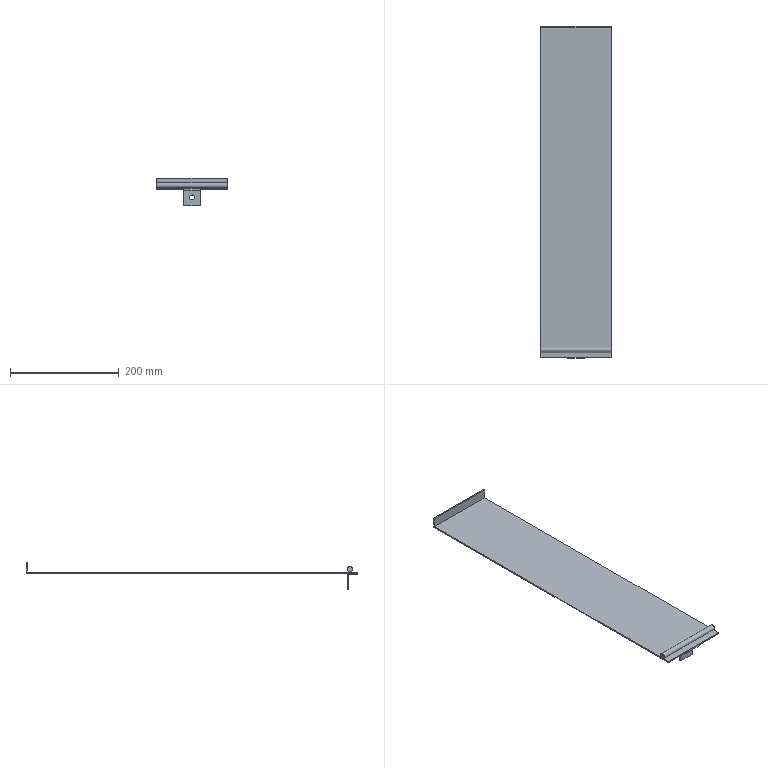Part | NX | features solid 2 | 1 solid | 17 faces | box 130 x 610 x 50 mm | volume 201020 mm3 | plane 15 | cylinder 2 | commonest cylinder face diameters 9 x1 10 x1
STEP:
#1=CARTESIAN_POINT('',(65.,-100.,-520.));
#2=VERTEX_POINT('',#1);
#3=CARTESIAN_POINT('',(65.,-710.,-520.));
#4=VERTEX_POINT('',#3);
#5=CARTESIAN_POINT('',(65.,20.,-520.));
#6=DIRECTION('',(0.,-1.,0.));
#7=VECTOR('',#6,1000.);
#8=LINE('',#5,#7);
#9=EDGE_CURVE('',#2,#4,#8,.T.);
#10=ORIENTED_EDGE('',*,*,#9,.F.);
#11=CARTESIAN_POINT('',(195.,-100.,-520.));
#12=VERTEX_POINT('',#11);
#13=CARTESIAN_POINT('',(365.,-100.,-520.));
#14=DIRECTION('',(1.,0.,0.));
#15=VECTOR('',#14,1000.);
#16=LINE('',#13,#15);
#17=EDGE_CURVE('',#12,#2,#16,.F.);
#18=ORIENTED_EDGE('',*,*,#17,.F.);
#19=CARTESIAN_POINT('',(195.,-710.,-520.));
#20=VERTEX_POINT('',#19);
#21=CARTESIAN_POINT('',(195.,-690.,-520.));
#22=DIRECTION('',(0.,-1.,0.));
#23=VECTOR('',#22,1000.);
#24=LINE('',#21,#23);
#25=EDGE_CURVE('',#12,#20,#24,.T.);
#26=ORIENTED_EDGE('',*,*,#25,.T.);
#27=CARTESIAN_POINT('',(145.,-710.,-520.));
#28=VERTEX_POINT('',#27);
#29=CARTESIAN_POINT('',(1630.,-710.,-520.));
#30=DIRECTION('',(-1.,0.,0.));
#31=VECTOR('',#30,1000.);
#32=LINE('',#29,#31);
#33=EDGE_CURVE('',#20,#28,#32,.T.);
#34=ORIENTED_EDGE('',*,*,#33,.T.);
#35=CARTESIAN_POINT('',(145.,-690.,-520.));
#36=VERTEX_POINT('',#35);
#37=CARTESIAN_POINT('',(145.,-690.,-520.));
#38=DIRECTION('',(0.,-1.,0.));
#39=VECTOR('',#38,1000.);
#40=LINE('',#37,#39);
#41=EDGE_CURVE('',#28,#36,#40,.F.);
#42=ORIENTED_EDGE('',*,*,#41,.T.);
#43=CARTESIAN_POINT('',(115.,-690.,-520.));
#44=VERTEX_POINT('',#43);
#45=CARTESIAN_POINT('',(155.,-690.,-520.));
#46=DIRECTION('',(-1.,0.,0.));
#47=VECTOR('',#46,1000.);
#48=LINE('',#45,#47);
#49=EDGE_CURVE('',#36,#44,#48,.T.);
#50=ORIENTED_EDGE('',*,*,#49,.T.);
#51=CARTESIAN_POINT('',(115.,-710.,-520.));
#52=VERTEX_POINT('',#51);
#53=CARTESIAN_POINT('',(115.,-690.,-520.));
#54=DIRECTION('',(0.,-1.,0.));
#55=VECTOR('',#54,1000.);
#56=LINE('',#53,#55);
#57=EDGE_CURVE('',#44,#52,#56,.T.);
#58=ORIENTED_EDGE('',*,*,#57,.T.);
#59=CARTESIAN_POINT('',(1630.,-710.,-520.));
#60=DIRECTION('',(-1.,0.,0.));
#61=VECTOR('',#60,1000.);
#62=LINE('',#59,#61);
#63=EDGE_CURVE('',#52,#4,#62,.T.);
#64=ORIENTED_EDGE('',*,*,#63,.T.);
#65=EDGE_LOOP('',(#10,#18,#26,#34,#42,#50,#58,#64));
#66=FACE_BOUND('',#65,.T.);
#67=CARTESIAN_POINT('',(365.,-10.,-520.));
#68=DIRECTION('',(0.,0.,-1.));
#69=DIRECTION('',(-1.,0.,0.));
#70=AXIS2_PLACEMENT_3D('',#67,#68,#69);
#71=PLANE('',#70);
#72=ADVANCED_FACE('',(#66),#71,.T.);
#73=CARTESIAN_POINT('',(65.,-102.3,-517.7));
#74=VERTEX_POINT('',#73);
#75=CARTESIAN_POINT('',(65.,-694.005,-517.7));
#76=VERTEX_POINT('',#75);
#77=CARTESIAN_POINT('',(65.,20.,-517.7));
#78=DIRECTION('',(0.,-1.,0.));
#79=VECTOR('',#78,1000.);
#80=LINE('',#77,#79);
#81=EDGE_CURVE('',#74,#76,#80,.T.);
#82=ORIENTED_EDGE('',*,*,#81,.F.);
#83=CARTESIAN_POINT('',(65.,-102.3,-500.));
#84=VERTEX_POINT('',#83);
#85=CARTESIAN_POINT('',(65.,-102.3,-520.));
#86=DIRECTION('',(0.,0.,-1.));
#87=VECTOR('',#86,1000.);
#88=LINE('',#85,#87);
#89=EDGE_CURVE('',#74,#84,#88,.F.);
#90=ORIENTED_EDGE('',*,*,#89,.T.);
#91=CARTESIAN_POINT('',(65.,-100.,-500.));
#92=VERTEX_POINT('',#91);
#93=CARTESIAN_POINT('',(65.,-92.3,-500.));
#94=DIRECTION('',(0.,1.,0.));
#95=VECTOR('',#94,1000.);
#96=LINE('',#93,#95);
#97=EDGE_CURVE('',#92,#84,#96,.F.);
#98=ORIENTED_EDGE('',*,*,#97,.F.);
#99=CARTESIAN_POINT('',(65.,-100.,-520.));
#100=DIRECTION('',(0.,0.,-1.));
#101=VECTOR('',#100,1000.);
#102=LINE('',#99,#101);
#103=EDGE_CURVE('',#2,#92,#102,.F.);
#104=ORIENTED_EDGE('',*,*,#103,.F.);
#105=ORIENTED_EDGE('',*,*,#9,.T.);
#106=CARTESIAN_POINT('',(65.,-710.,-517.7));
#107=VERTEX_POINT('',#106);
#108=CARTESIAN_POINT('',(65.,-710.,-520.));
#109=DIRECTION('',(0.,0.,1.));
#110=VECTOR('',#109,1000.);
#111=LINE('',#108,#110);
#112=EDGE_CURVE('',#4,#107,#111,.T.);
#113=ORIENTED_EDGE('',*,*,#112,.T.);
#114=CARTESIAN_POINT('',(65.,-695.995,-517.7));
#115=VERTEX_POINT('',#114);
#116=CARTESIAN_POINT('',(65.,20.,-517.7));
#117=DIRECTION('',(0.,-1.,0.));
#118=VECTOR('',#117,1000.);
#119=LINE('',#116,#118);
#120=EDGE_CURVE('',#115,#107,#119,.T.);
#121=ORIENTED_EDGE('',*,*,#120,.F.);
#122=CARTESIAN_POINT('',(65.,-695.,-512.8));
#123=DIRECTION('',(-1.,0.,0.));
#124=DIRECTION('',(0.,0.,1.));
#125=AXIS2_PLACEMENT_3D('',#122,#123,#124);
#126=CIRCLE('',#125,5.);
#127=EDGE_CURVE('',#76,#115,#126,.F.);
#128=ORIENTED_EDGE('',*,*,#127,.F.);
#129=EDGE_LOOP('',(#82,#90,#98,#104,#105,#113,#121,#128));
#130=FACE_BOUND('',#129,.T.);
#131=CARTESIAN_POINT('',(65.,20.,-520.));
#132=DIRECTION('',(-1.,0.,0.));
#133=DIRECTION('',(0.,0.,1.));
#134=AXIS2_PLACEMENT_3D('',#131,#132,#133);
#135=PLANE('',#134);
#136=ADVANCED_FACE('',(#130),#135,.T.);
#137=ORIENTED_EDGE('',*,*,#81,.T.);
#138=CARTESIAN_POINT('',(195.,-694.005,-517.7));
#139=VERTEX_POINT('',#138);
#140=CARTESIAN_POINT('',(130.,-694.005,-517.7));
#141=DIRECTION('',(1.,0.,0.));
#142=VECTOR('',#141,1000.);
#143=LINE('',#140,#142);
#144=EDGE_CURVE('',#139,#76,#143,.F.);
#145=ORIENTED_EDGE('',*,*,#144,.F.);
#146=CARTESIAN_POINT('',(195.,-102.3,-517.7));
#147=VERTEX_POINT('',#146);
#148=CARTESIAN_POINT('',(195.,-690.,-517.7));
#149=DIRECTION('',(0.,-1.,0.));
#150=VECTOR('',#149,1000.);
#151=LINE('',#148,#150);
#152=EDGE_CURVE('',#147,#139,#151,.T.);
#153=ORIENTED_EDGE('',*,*,#152,.F.);
#154=CARTESIAN_POINT('',(646.442,-102.3,-517.7));
#155=DIRECTION('',(1.,0.,0.));
#156=VECTOR('',#155,1000.);
#157=LINE('',#154,#156);
#158=EDGE_CURVE('',#147,#74,#157,.F.);
#159=ORIENTED_EDGE('',*,*,#158,.T.);
#160=EDGE_LOOP('',(#137,#145,#153,#159));
#161=FACE_BOUND('',#160,.T.);
#162=CARTESIAN_POINT('',(1630.,10.,-517.7));
#163=DIRECTION('',(0.,0.,-1.));
#164=DIRECTION('',(1.,0.,0.));
#165=AXIS2_PLACEMENT_3D('',#162,#163,#164);
#166=PLANE('',#165);
#167=ADVANCED_FACE('',(#161),#166,.F.);
#168=ORIENTED_EDGE('',*,*,#25,.F.);
#169=CARTESIAN_POINT('',(195.,-100.,-500.));
#170=VERTEX_POINT('',#169);
#171=CARTESIAN_POINT('',(195.,-100.,-520.));
#172=DIRECTION('',(0.,0.,-1.));
#173=VECTOR('',#172,1000.);
#174=LINE('',#171,#173);
#175=EDGE_CURVE('',#12,#170,#174,.F.);
#176=ORIENTED_EDGE('',*,*,#175,.T.);
#177=CARTESIAN_POINT('',(195.,-102.3,-500.));
#178=VERTEX_POINT('',#177);
#179=CARTESIAN_POINT('',(195.,-690.,-500.));
#180=DIRECTION('',(0.,-1.,0.));
#181=VECTOR('',#180,1000.);
#182=LINE('',#179,#181);
#183=EDGE_CURVE('',#178,#170,#182,.F.);
#184=ORIENTED_EDGE('',*,*,#183,.F.);
#185=CARTESIAN_POINT('',(195.,-102.3,-382.7));
#186=DIRECTION('',(0.,0.,-1.));
#187=VECTOR('',#186,1000.);
#188=LINE('',#185,#187);
#189=EDGE_CURVE('',#147,#178,#188,.F.);
#190=ORIENTED_EDGE('',*,*,#189,.F.);
#191=ORIENTED_EDGE('',*,*,#152,.T.);
#192=CARTESIAN_POINT('',(195.,-695.995,-517.7));
#193=VERTEX_POINT('',#192);
#194=CARTESIAN_POINT('',(195.,-695.,-512.8));
#195=DIRECTION('',(-1.,0.,0.));
#196=DIRECTION('',(0.,0.,1.));
#197=AXIS2_PLACEMENT_3D('',#194,#195,#196);
#198=CIRCLE('',#197,5.);
#199=EDGE_CURVE('',#193,#139,#198,.T.);
#200=ORIENTED_EDGE('',*,*,#199,.F.);
#201=CARTESIAN_POINT('',(195.,-710.,-517.7));
#202=VERTEX_POINT('',#201);
#203=CARTESIAN_POINT('',(195.,-690.,-517.7));
#204=DIRECTION('',(0.,-1.,0.));
#205=VECTOR('',#204,1000.);
#206=LINE('',#203,#205);
#207=EDGE_CURVE('',#193,#202,#206,.T.);
#208=ORIENTED_EDGE('',*,*,#207,.T.);
#209=CARTESIAN_POINT('',(195.,-710.,-382.7));
#210=DIRECTION('',(0.,0.,1.));
#211=VECTOR('',#210,1000.);
#212=LINE('',#209,#211);
#213=EDGE_CURVE('',#20,#202,#212,.T.);
#214=ORIENTED_EDGE('',*,*,#213,.F.);
#215=EDGE_LOOP('',(#168,#176,#184,#190,#191,#200,#208,#214));
#216=FACE_BOUND('',#215,.T.);
#217=CARTESIAN_POINT('',(195.,-690.,-382.7));
#218=DIRECTION('',(-1.,0.,0.));
#219=DIRECTION('',(0.,0.,-1.));
#220=AXIS2_PLACEMENT_3D('',#217,#218,#219);
#221=PLANE('',#220);
#222=ADVANCED_FACE('',(#216),#221,.F.);
#223=CARTESIAN_POINT('',(365.,-695.995,-517.7));
#224=DIRECTION('',(1.,0.,0.));
#225=VECTOR('',#224,1000.);
#226=LINE('',#223,#225);
#227=EDGE_CURVE('',#115,#193,#226,.T.);
#228=ORIENTED_EDGE('',*,*,#227,.F.);
#229=ORIENTED_EDGE('',*,*,#120,.T.);
#230=CARTESIAN_POINT('',(1630.,-710.,-517.7));
#231=DIRECTION('',(-1.,0.,0.));
#232=VECTOR('',#231,1000.);
#233=LINE('',#230,#232);
#234=EDGE_CURVE('',#202,#107,#233,.T.);
#235=ORIENTED_EDGE('',*,*,#234,.F.);
#236=ORIENTED_EDGE('',*,*,#207,.F.);
#237=EDGE_LOOP('',(#228,#229,#235,#236));
#238=FACE_BOUND('',#237,.T.);
#239=CARTESIAN_POINT('',(1630.,-20.,-517.7));
#240=DIRECTION('',(0.,0.,-1.));
#241=DIRECTION('',(1.,0.,0.));
#242=AXIS2_PLACEMENT_3D('',#239,#240,#241);
#243=PLANE('',#242);
#244=ADVANCED_FACE('',(#238),#243,.F.);
#245=ORIENTED_EDGE('',*,*,#213,.T.);
#246=ORIENTED_EDGE('',*,*,#234,.T.);
#247=ORIENTED_EDGE('',*,*,#112,.F.);
#248=ORIENTED_EDGE('',*,*,#63,.F.);
#249=CARTESIAN_POINT('',(115.,-710.,-522.3));
#250=VERTEX_POINT('',#249);
#251=CARTESIAN_POINT('',(115.,-710.,-520.));
#252=DIRECTION('',(0.,0.,-1.));
#253=VECTOR('',#252,1000.);
#254=LINE('',#251,#253);
#255=EDGE_CURVE('',#52,#250,#254,.T.);
#256=ORIENTED_EDGE('',*,*,#255,.T.);
#257=CARTESIAN_POINT('',(145.,-710.,-522.3));
#258=VERTEX_POINT('',#257);
#259=CARTESIAN_POINT('',(1542.5,-710.,-522.3));
#260=DIRECTION('',(1.,0.,0.));
#261=VECTOR('',#260,1000.);
#262=LINE('',#259,#261);
#263=EDGE_CURVE('',#258,#250,#262,.F.);
#264=ORIENTED_EDGE('',*,*,#263,.F.);
#265=CARTESIAN_POINT('',(145.,-710.,-520.));
#266=DIRECTION('',(0.,0.,1.));
#267=VECTOR('',#266,1000.);
#268=LINE('',#265,#267);
#269=EDGE_CURVE('',#28,#258,#268,.F.);
#270=ORIENTED_EDGE('',*,*,#269,.F.);
#271=ORIENTED_EDGE('',*,*,#33,.F.);
#272=EDGE_LOOP('',(#245,#246,#247,#248,#256,#264,#270,#271));
#273=FACE_BOUND('',#272,.T.);
#274=CARTESIAN_POINT('',(1630.,-710.,-520.));
#275=DIRECTION('',(0.,-1.,0.));
#276=DIRECTION('',(0.,0.,-1.));
#277=AXIS2_PLACEMENT_3D('',#274,#275,#276);
#278=PLANE('',#277);
#279=ADVANCED_FACE('',(#273),#278,.T.);
#280=ORIENTED_EDGE('',*,*,#199,.T.);
#281=ORIENTED_EDGE('',*,*,#144,.T.);
#282=ORIENTED_EDGE('',*,*,#127,.T.);
#283=ORIENTED_EDGE('',*,*,#227,.T.);
#284=EDGE_LOOP('',(#280,#281,#282,#283));
#285=FACE_BOUND('',#284,.T.);
#286=CARTESIAN_POINT('',(365.,-695.,-512.8));
#287=DIRECTION('',(1.,0.,0.));
#288=DIRECTION('',(0.,0.,1.));
#289=AXIS2_PLACEMENT_3D('',#286,#287,#288);
#290=CYLINDRICAL_SURFACE('',#289,5.);
#291=ADVANCED_FACE('',(#285),#290,.T.);
#292=CARTESIAN_POINT('',(130.,-692.3,-530.5));
#293=VERTEX_POINT('',#292);
#294=CARTESIAN_POINT('',(130.,-692.3,-535.));
#295=DIRECTION('',(0.,-1.,0.));
#296=DIRECTION('',(0.,0.,1.));
#297=AXIS2_PLACEMENT_3D('',#294,#295,#296);
#298=CIRCLE('',#297,4.5);
#299=EDGE_CURVE('',#293,#293,#298,.T.);
#300=ORIENTED_EDGE('',*,*,#299,.F.);
#301=EDGE_LOOP('',(#300));
#302=FACE_BOUND('',#301,.T.);
#303=CARTESIAN_POINT('',(145.,-692.3,-522.3));
#304=VERTEX_POINT('',#303);
#305=CARTESIAN_POINT('',(115.,-692.3,-522.3));
#306=VERTEX_POINT('',#305);
#307=CARTESIAN_POINT('',(155.,-692.3,-522.3));
#308=DIRECTION('',(-1.,0.,0.));
#309=VECTOR('',#308,1000.);
#310=LINE('',#307,#309);
#311=EDGE_CURVE('',#304,#306,#310,.T.);
#312=ORIENTED_EDGE('',*,*,#311,.T.);
#313=CARTESIAN_POINT('',(115.,-692.3,-550.));
#314=VERTEX_POINT('',#313);
#315=CARTESIAN_POINT('',(115.,-692.3,-520.));
#316=DIRECTION('',(0.,0.,-1.));
#317=VECTOR('',#316,1000.);
#318=LINE('',#315,#317);
#319=EDGE_CURVE('',#306,#314,#318,.T.);
#320=ORIENTED_EDGE('',*,*,#319,.T.);
#321=CARTESIAN_POINT('',(145.,-692.3,-550.));
#322=VERTEX_POINT('',#321);
#323=CARTESIAN_POINT('',(155.,-692.3,-550.));
#324=DIRECTION('',(1.,0.,0.));
#325=VECTOR('',#324,1000.);
#326=LINE('',#323,#325);
#327=EDGE_CURVE('',#322,#314,#326,.F.);
#328=ORIENTED_EDGE('',*,*,#327,.F.);
#329=CARTESIAN_POINT('',(145.,-692.3,-520.));
#330=DIRECTION('',(0.,0.,1.));
#331=VECTOR('',#330,1000.);
#332=LINE('',#329,#331);
#333=EDGE_CURVE('',#304,#322,#332,.F.);
#334=ORIENTED_EDGE('',*,*,#333,.F.);
#335=EDGE_LOOP('',(#312,#320,#328,#334));
#336=FACE_BOUND('',#335,.T.);
#337=CARTESIAN_POINT('',(155.,-692.3,-520.));
#338=DIRECTION('',(0.,1.,0.));
#339=DIRECTION('',(0.,0.,1.));
#340=AXIS2_PLACEMENT_3D('',#337,#338,#339);
#341=PLANE('',#340);
#342=ADVANCED_FACE('',(#302,#336),#341,.F.);
#343=CARTESIAN_POINT('',(145.,-745.,-522.3));
#344=DIRECTION('',(0.,1.,0.));
#345=VECTOR('',#344,1000.);
#346=LINE('',#343,#345);
#347=EDGE_CURVE('',#258,#304,#346,.T.);
#348=ORIENTED_EDGE('',*,*,#347,.F.);
#349=ORIENTED_EDGE('',*,*,#263,.T.);
#350=CARTESIAN_POINT('',(115.,-690.,-522.3));
#351=DIRECTION('',(0.,-1.,0.));
#352=VECTOR('',#351,1000.);
#353=LINE('',#350,#352);
#354=EDGE_CURVE('',#250,#306,#353,.F.);
#355=ORIENTED_EDGE('',*,*,#354,.T.);
#356=ORIENTED_EDGE('',*,*,#311,.F.);
#357=EDGE_LOOP('',(#348,#349,#355,#356));
#358=FACE_BOUND('',#357,.T.);
#359=CARTESIAN_POINT('',(277.5,-745.,-522.3));
#360=DIRECTION('',(0.,0.,1.));
#361=DIRECTION('',(-1.,0.,0.));
#362=AXIS2_PLACEMENT_3D('',#359,#360,#361);
#363=PLANE('',#362);
#364=ADVANCED_FACE('',(#358),#363,.F.);
#365=CARTESIAN_POINT('',(130.,-690.,-530.5));
#366=VERTEX_POINT('',#365);
#367=CARTESIAN_POINT('',(130.,-690.,-535.));
#368=DIRECTION('',(0.,-1.,0.));
#369=DIRECTION('',(0.,0.,1.));
#370=AXIS2_PLACEMENT_3D('',#367,#368,#369);
#371=CIRCLE('',#370,4.5);
#372=EDGE_CURVE('',#366,#366,#371,.T.);
#373=ORIENTED_EDGE('',*,*,#372,.F.);
#374=EDGE_LOOP('',(#373));
#375=FACE_BOUND('',#374,.T.);
#376=ORIENTED_EDGE('',*,*,#299,.T.);
#377=EDGE_LOOP('',(#376));
#378=FACE_BOUND('',#377,.T.);
#379=CARTESIAN_POINT('',(130.,-692.3,-535.));
#380=DIRECTION('',(0.,1.,0.));
#381=DIRECTION('',(0.,0.,1.));
#382=AXIS2_PLACEMENT_3D('',#379,#380,#381);
#383=CYLINDRICAL_SURFACE('',#382,4.5);
#384=ADVANCED_FACE('',(#375,#378),#383,.F.);
#385=CARTESIAN_POINT('',(145.,-690.,-550.));
#386=VERTEX_POINT('',#385);
#387=CARTESIAN_POINT('',(145.,-690.,-550.));
#388=DIRECTION('',(0.,-1.,0.));
#389=VECTOR('',#388,1000.);
#390=LINE('',#387,#389);
#391=EDGE_CURVE('',#386,#322,#390,.T.);
#392=ORIENTED_EDGE('',*,*,#391,.T.);
#393=ORIENTED_EDGE('',*,*,#327,.T.);
#394=CARTESIAN_POINT('',(115.,-690.,-550.));
#395=VERTEX_POINT('',#394);
#396=CARTESIAN_POINT('',(115.,-690.,-550.));
#397=DIRECTION('',(0.,1.,0.));
#398=VECTOR('',#397,1000.);
#399=LINE('',#396,#398);
#400=EDGE_CURVE('',#395,#314,#399,.F.);
#401=ORIENTED_EDGE('',*,*,#400,.F.);
#402=CARTESIAN_POINT('',(155.,-690.,-550.));
#403=DIRECTION('',(1.,0.,0.));
#404=VECTOR('',#403,1000.);
#405=LINE('',#402,#404);
#406=EDGE_CURVE('',#386,#395,#405,.F.);
#407=ORIENTED_EDGE('',*,*,#406,.F.);
#408=EDGE_LOOP('',(#392,#393,#401,#407));
#409=FACE_BOUND('',#408,.T.);
#410=CARTESIAN_POINT('',(155.,-690.,-550.));
#411=DIRECTION('',(0.,0.,1.));
#412=DIRECTION('',(-1.,0.,0.));
#413=AXIS2_PLACEMENT_3D('',#410,#411,#412);
#414=PLANE('',#413);
#415=ADVANCED_FACE('',(#409),#414,.F.);
#416=CARTESIAN_POINT('',(115.,-690.,-520.));
#417=DIRECTION('',(0.,0.,-1.));
#418=VECTOR('',#417,1000.);
#419=LINE('',#416,#418);
#420=EDGE_CURVE('',#44,#395,#419,.T.);
#421=ORIENTED_EDGE('',*,*,#420,.F.);
#422=ORIENTED_EDGE('',*,*,#49,.F.);
#423=CARTESIAN_POINT('',(145.,-690.,-520.));
#424=DIRECTION('',(0.,0.,1.));
#425=VECTOR('',#424,1000.);
#426=LINE('',#423,#425);
#427=EDGE_CURVE('',#36,#386,#426,.F.);
#428=ORIENTED_EDGE('',*,*,#427,.T.);
#429=ORIENTED_EDGE('',*,*,#406,.T.);
#430=EDGE_LOOP('',(#421,#422,#428,#429));
#431=FACE_BOUND('',#430,.T.);
#432=ORIENTED_EDGE('',*,*,#372,.T.);
#433=EDGE_LOOP('',(#432));
#434=FACE_BOUND('',#433,.T.);
#435=CARTESIAN_POINT('',(155.,-690.,-520.));
#436=DIRECTION('',(0.,1.,0.));
#437=DIRECTION('',(0.,0.,1.));
#438=AXIS2_PLACEMENT_3D('',#435,#436,#437);
#439=PLANE('',#438);
#440=ADVANCED_FACE('',(#431,#434),#439,.T.);
#441=ORIENTED_EDGE('',*,*,#354,.F.);
#442=ORIENTED_EDGE('',*,*,#255,.F.);
#443=ORIENTED_EDGE('',*,*,#57,.F.);
#444=ORIENTED_EDGE('',*,*,#420,.T.);
#445=ORIENTED_EDGE('',*,*,#400,.T.);
#446=ORIENTED_EDGE('',*,*,#319,.F.);
#447=EDGE_LOOP('',(#441,#442,#443,#444,#445,#446));
#448=FACE_BOUND('',#447,.T.);
#449=CARTESIAN_POINT('',(115.,-690.,-520.));
#450=DIRECTION('',(-1.,0.,0.));
#451=DIRECTION('',(0.,0.,-1.));
#452=AXIS2_PLACEMENT_3D('',#449,#450,#451);
#453=PLANE('',#452);
#454=ADVANCED_FACE('',(#448),#453,.T.);
#455=ORIENTED_EDGE('',*,*,#427,.F.);
#456=ORIENTED_EDGE('',*,*,#41,.F.);
#457=ORIENTED_EDGE('',*,*,#269,.T.);
#458=ORIENTED_EDGE('',*,*,#347,.T.);
#459=ORIENTED_EDGE('',*,*,#333,.T.);
#460=ORIENTED_EDGE('',*,*,#391,.F.);
#461=EDGE_LOOP('',(#455,#456,#457,#458,#459,#460));
#462=FACE_BOUND('',#461,.T.);
#463=CARTESIAN_POINT('',(145.,-690.,-520.));
#464=DIRECTION('',(-1.,0.,0.));
#465=DIRECTION('',(0.,0.,-1.));
#466=AXIS2_PLACEMENT_3D('',#463,#464,#465);
#467=PLANE('',#466);
#468=ADVANCED_FACE('',(#462),#467,.F.);
#469=ORIENTED_EDGE('',*,*,#17,.T.);
#470=ORIENTED_EDGE('',*,*,#103,.T.);
#471=CARTESIAN_POINT('',(365.,-100.,-500.));
#472=DIRECTION('',(-1.,0.,0.));
#473=VECTOR('',#472,1000.);
#474=LINE('',#471,#473);
#475=EDGE_CURVE('',#170,#92,#474,.T.);
#476=ORIENTED_EDGE('',*,*,#475,.F.);
#477=ORIENTED_EDGE('',*,*,#175,.F.);
#478=EDGE_LOOP('',(#469,#470,#476,#477));
#479=FACE_BOUND('',#478,.T.);
#480=CARTESIAN_POINT('',(365.,-100.,-520.));
#481=DIRECTION('',(0.,-1.,0.));
#482=DIRECTION('',(0.,0.,-1.));
#483=AXIS2_PLACEMENT_3D('',#480,#481,#482);
#484=PLANE('',#483);
#485=ADVANCED_FACE('',(#479),#484,.F.);
#486=ORIENTED_EDGE('',*,*,#183,.T.);
#487=ORIENTED_EDGE('',*,*,#475,.T.);
#488=ORIENTED_EDGE('',*,*,#97,.T.);
#489=CARTESIAN_POINT('',(365.,-102.3,-500.));
#490=DIRECTION('',(-1.,0.,0.));
#491=VECTOR('',#490,1000.);
#492=LINE('',#489,#491);
#493=EDGE_CURVE('',#178,#84,#492,.T.);
#494=ORIENTED_EDGE('',*,*,#493,.F.);
#495=EDGE_LOOP('',(#486,#487,#488,#494));
#496=FACE_BOUND('',#495,.T.);
#497=CARTESIAN_POINT('',(365.,-92.3,-500.));
#498=DIRECTION('',(0.,0.,-1.));
#499=DIRECTION('',(-1.,0.,0.));
#500=AXIS2_PLACEMENT_3D('',#497,#498,#499);
#501=PLANE('',#500);
#502=ADVANCED_FACE('',(#496),#501,.F.);
#503=ORIENTED_EDGE('',*,*,#189,.T.);
#504=ORIENTED_EDGE('',*,*,#493,.T.);
#505=ORIENTED_EDGE('',*,*,#89,.F.);
#506=ORIENTED_EDGE('',*,*,#158,.F.);
#507=EDGE_LOOP('',(#503,#504,#505,#506));
#508=FACE_BOUND('',#507,.T.);
#509=CARTESIAN_POINT('',(646.442,-102.3,-247.7));
#510=DIRECTION('',(0.,1.,0.));
#511=DIRECTION('',(0.,0.,1.));
#512=AXIS2_PLACEMENT_3D('',#509,#510,#511);
#513=PLANE('',#512);
#514=ADVANCED_FACE('',(#508),#513,.F.);
#515=CLOSED_SHELL('',(#72,#136,#167,#222,#244,#279,#291,#342,#364,#384,#415,#440,#454,#468,#485,#502,#514));
#516=MANIFOLD_SOLID_BREP('',#515);
#517=(LENGTH_UNIT()NAMED_UNIT(*)SI_UNIT(.MILLI.,.METRE.));
#518=UNCERTAINTY_MEASURE_WITH_UNIT(LENGTH_MEASURE(0.00001),#517,'','');
#519=(NAMED_UNIT(*)PLANE_ANGLE_UNIT()SI_UNIT($,.RADIAN.));
#520=(NAMED_UNIT(*)SI_UNIT($,.STERADIAN.)SOLID_ANGLE_UNIT());
#521=(GEOMETRIC_REPRESENTATION_CONTEXT(3)GLOBAL_UNCERTAINTY_ASSIGNED_CONTEXT((#518))GLOBAL_UNIT_ASSIGNED_CONTEXT((#517,#519,#520))REPRESENTATION_CONTEXT('',''));
#522=ADVANCED_BREP_SHAPE_REPRESENTATION('',(#516),#521);